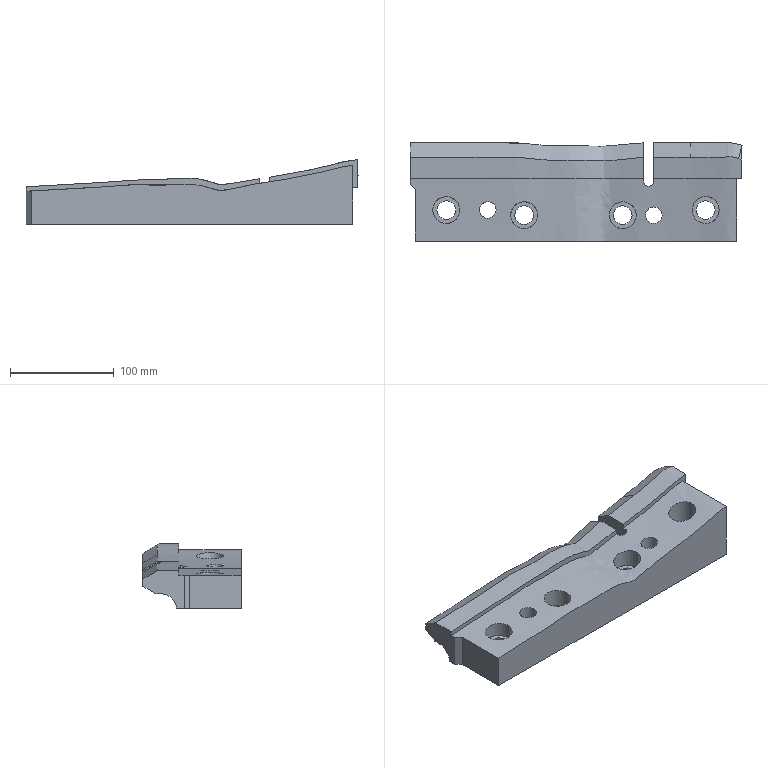Part | NX | features solid 2 | 1 solid | 55 faces | box 320 x 94.748 x 62.253 mm | volume 888954 mm3 | spline 25 | plane 19 | cylinder 11 | commonest cylinder face diameters 18 x4 26 x4 16 x2 10 x1